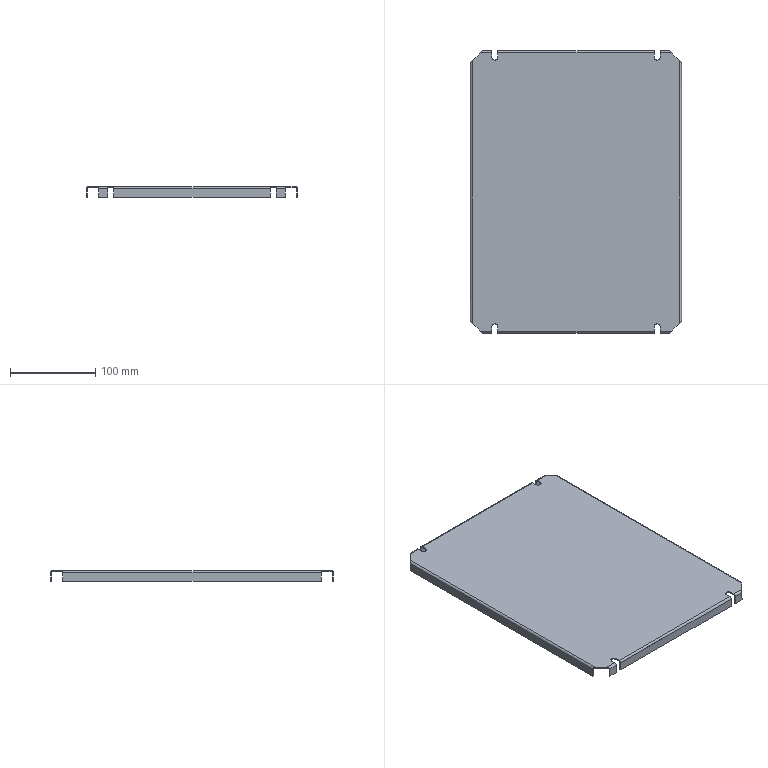Part | SolidWorks | features BaseBody 1 | 1 solid | 74 faces | box 248 x 332 x 12.6 mm | volume 110968 mm3 | plane 46 | cylinder 20 | spline 8 | commonest cylinder face diameters 2.4 x8 4.8 x8 7 x4